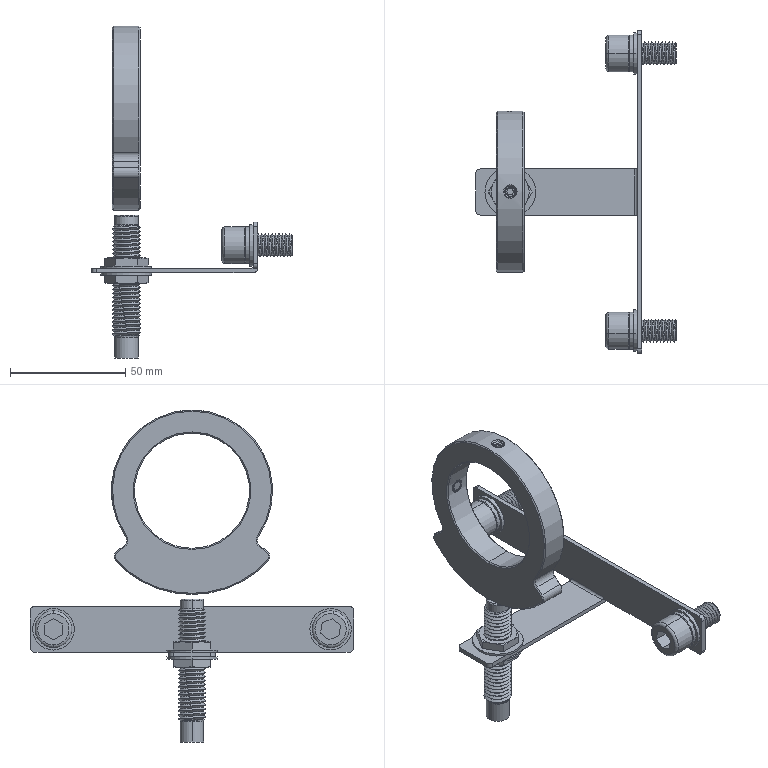Part | SolidWorks | 9 solids | 425 faces | box 87 x 140.21 x 144 mm | volume 53103 mm3 | cylinder 224 | plane 92 | cone 64 | spline 34 | torus 11 | commonest cylinder face diameters 12 x65 10 x50 4 x41 6 x36 10.2 x10 16 x8